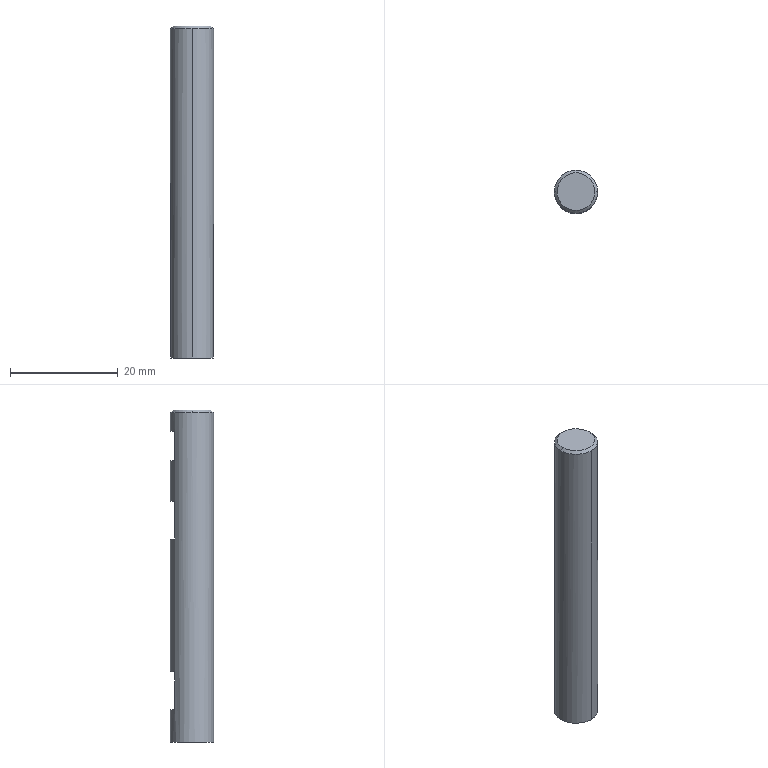Part | NX | 1 solid | 23 faces | box 8 x 8 x 61.5 mm | volume 2929 mm3 | plane 11 | cylinder 6 | cone 6 | commonest cylinder face diameters 3.3 x4 8 x2
STEP:
#1=CARTESIAN_POINT('',(-190.,192.7,-6.3));
#2=VERTEX_POINT('',#1);
#3=CARTESIAN_POINT('',(-194.,196.7,-6.3));
#4=VERTEX_POINT('',#3);
#5=CARTESIAN_POINT('',(-190.,196.7,-6.3));
#6=DIRECTION('',(0.,0.,-1.));
#7=DIRECTION('',(-1.,0.,0.));
#8=AXIS2_PLACEMENT_3D('',#5,#6,#7);
#9=CIRCLE('',#8,4.);
#10=EDGE_CURVE('',#2,#4,#9,.T.);
#11=ORIENTED_EDGE('',*,*,#10,.T.);
#12=CARTESIAN_POINT('',(-190.,200.7,-6.3));
#13=VERTEX_POINT('',#12);
#14=CARTESIAN_POINT('',(-190.,196.7,-6.3));
#15=DIRECTION('',(0.,0.,-1.));
#16=DIRECTION('',(-1.,0.,0.));
#17=AXIS2_PLACEMENT_3D('',#14,#15,#16);
#18=CIRCLE('',#17,4.);
#19=EDGE_CURVE('',#4,#13,#18,.T.);
#20=ORIENTED_EDGE('',*,*,#19,.T.);
#21=CARTESIAN_POINT('',(-190.,200.7,-9.7));
#22=VERTEX_POINT('',#21);
#23=CARTESIAN_POINT('',(-190.,200.7,-55.8));
#24=DIRECTION('',(0.,0.,1.));
#25=VECTOR('',#24,1000.);
#26=LINE('',#23,#25);
#27=EDGE_CURVE('',#13,#22,#26,.F.);
#28=ORIENTED_EDGE('',*,*,#27,.T.);
#29=CARTESIAN_POINT('',(-192.4,199.9,-9.7));
#30=VERTEX_POINT('',#29);
#31=CARTESIAN_POINT('',(-190.,196.7,-9.7));
#32=DIRECTION('',(0.,0.,1.));
#33=DIRECTION('',(0.,-1.,0.));
#34=AXIS2_PLACEMENT_3D('',#31,#32,#33);
#35=CIRCLE('',#34,4.);
#36=EDGE_CURVE('',#22,#30,#35,.T.);
#37=ORIENTED_EDGE('',*,*,#36,.T.);
#38=CARTESIAN_POINT('',(-192.4,199.9,-15.2));
#39=VERTEX_POINT('',#38);
#40=CARTESIAN_POINT('',(-192.4,199.9,-55.8));
#41=DIRECTION('',(0.,0.,1.));
#42=VECTOR('',#41,1000.);
#43=LINE('',#40,#42);
#44=EDGE_CURVE('',#39,#30,#43,.T.);
#45=ORIENTED_EDGE('',*,*,#44,.F.);
#46=CARTESIAN_POINT('',(-190.,200.7,-15.2));
#47=VERTEX_POINT('',#46);
#48=CARTESIAN_POINT('',(-190.,196.7,-15.2));
#49=DIRECTION('',(0.,0.,1.));
#50=DIRECTION('',(0.,-1.,0.));
#51=AXIS2_PLACEMENT_3D('',#48,#49,#50);
#52=CIRCLE('',#51,4.);
#53=EDGE_CURVE('',#47,#39,#52,.T.);
#54=ORIENTED_EDGE('',*,*,#53,.F.);
#55=CARTESIAN_POINT('',(-190.,200.7,-22.7));
#56=VERTEX_POINT('',#55);
#57=CARTESIAN_POINT('',(-190.,200.7,-55.8));
#58=DIRECTION('',(0.,0.,1.));
#59=VECTOR('',#58,1000.);
#60=LINE('',#57,#59);
#61=EDGE_CURVE('',#56,#47,#60,.T.);
#62=ORIENTED_EDGE('',*,*,#61,.F.);
#63=CARTESIAN_POINT('',(-192.4,199.9,-22.7));
#64=VERTEX_POINT('',#63);
#65=CARTESIAN_POINT('',(-190.,196.7,-22.7));
#66=DIRECTION('',(0.,0.,1.));
#67=DIRECTION('',(0.,-1.,0.));
#68=AXIS2_PLACEMENT_3D('',#65,#66,#67);
#69=CIRCLE('',#68,4.);
#70=EDGE_CURVE('',#56,#64,#69,.T.);
#71=ORIENTED_EDGE('',*,*,#70,.T.);
#72=CARTESIAN_POINT('',(-192.4,199.9,-29.7));
#73=VERTEX_POINT('',#72);
#74=CARTESIAN_POINT('',(-192.4,199.9,-55.8));
#75=DIRECTION('',(0.,0.,1.));
#76=VECTOR('',#75,1000.);
#77=LINE('',#74,#76);
#78=EDGE_CURVE('',#73,#64,#77,.T.);
#79=ORIENTED_EDGE('',*,*,#78,.F.);
#80=CARTESIAN_POINT('',(-190.,200.7,-29.7));
#81=VERTEX_POINT('',#80);
#82=CARTESIAN_POINT('',(-190.,196.7,-29.7));
#83=DIRECTION('',(0.,0.,1.));
#84=DIRECTION('',(0.,-1.,0.));
#85=AXIS2_PLACEMENT_3D('',#82,#83,#84);
#86=CIRCLE('',#85,4.);
#87=EDGE_CURVE('',#81,#73,#86,.T.);
#88=ORIENTED_EDGE('',*,*,#87,.F.);
#89=CARTESIAN_POINT('',(-190.,200.7,-54.3));
#90=VERTEX_POINT('',#89);
#91=CARTESIAN_POINT('',(-190.,200.7,-55.8));
#92=DIRECTION('',(0.,0.,1.));
#93=VECTOR('',#92,1000.);
#94=LINE('',#91,#93);
#95=EDGE_CURVE('',#90,#81,#94,.T.);
#96=ORIENTED_EDGE('',*,*,#95,.F.);
#97=CARTESIAN_POINT('',(-192.4,199.9,-54.3));
#98=VERTEX_POINT('',#97);
#99=CARTESIAN_POINT('',(-190.,196.7,-54.3));
#100=DIRECTION('',(0.,0.,1.));
#101=DIRECTION('',(0.,-1.,0.));
#102=AXIS2_PLACEMENT_3D('',#99,#100,#101);
#103=CIRCLE('',#102,4.);
#104=EDGE_CURVE('',#90,#98,#103,.T.);
#105=ORIENTED_EDGE('',*,*,#104,.T.);
#106=CARTESIAN_POINT('',(-192.4,199.9,-61.3));
#107=VERTEX_POINT('',#106);
#108=CARTESIAN_POINT('',(-192.4,199.9,-55.8));
#109=DIRECTION('',(0.,0.,1.));
#110=VECTOR('',#109,1000.);
#111=LINE('',#108,#110);
#112=EDGE_CURVE('',#107,#98,#111,.T.);
#113=ORIENTED_EDGE('',*,*,#112,.F.);
#114=CARTESIAN_POINT('',(-190.,200.7,-61.3));
#115=VERTEX_POINT('',#114);
#116=CARTESIAN_POINT('',(-190.,196.7,-61.3));
#117=DIRECTION('',(0.,0.,1.));
#118=DIRECTION('',(0.,-1.,0.));
#119=AXIS2_PLACEMENT_3D('',#116,#117,#118);
#120=CIRCLE('',#119,4.);
#121=EDGE_CURVE('',#115,#107,#120,.T.);
#122=ORIENTED_EDGE('',*,*,#121,.F.);
#123=CARTESIAN_POINT('',(-190.,200.7,-67.3));
#124=VERTEX_POINT('',#123);
#125=CARTESIAN_POINT('',(-190.,200.7,-55.8));
#126=DIRECTION('',(0.,0.,1.));
#127=VECTOR('',#126,1000.);
#128=LINE('',#125,#127);
#129=EDGE_CURVE('',#124,#115,#128,.T.);
#130=ORIENTED_EDGE('',*,*,#129,.F.);
#131=CARTESIAN_POINT('',(-190.,192.7,-67.3));
#132=VERTEX_POINT('',#131);
#133=CARTESIAN_POINT('',(-190.,196.7,-67.3));
#134=DIRECTION('',(0.,0.,1.));
#135=DIRECTION('',(0.,-1.,0.));
#136=AXIS2_PLACEMENT_3D('',#133,#134,#135);
#137=CIRCLE('',#136,4.);
#138=EDGE_CURVE('',#124,#132,#137,.T.);
#139=ORIENTED_EDGE('',*,*,#138,.T.);
#140=CARTESIAN_POINT('',(-190.,192.7,-55.8));
#141=DIRECTION('',(0.,0.,1.));
#142=VECTOR('',#141,1000.);
#143=LINE('',#140,#142);
#144=EDGE_CURVE('',#2,#132,#143,.F.);
#145=ORIENTED_EDGE('',*,*,#144,.F.);
#146=EDGE_LOOP('',(#11,#20,#28,#37,#45,#54,#62,#71,#79,#88,#96,#105,#113,#122,#130,#139,#145));
#147=FACE_BOUND('',#146,.T.);
#148=CARTESIAN_POINT('',(-190.,196.7,-55.8));
#149=DIRECTION('',(0.,0.,1.));
#150=DIRECTION('',(0.,-1.,0.));
#151=AXIS2_PLACEMENT_3D('',#148,#149,#150);
#152=CYLINDRICAL_SURFACE('',#151,4.);
#153=ADVANCED_FACE('',(#147),#152,.T.);
#154=CARTESIAN_POINT('',(-193.5,196.7,-5.8));
#155=VERTEX_POINT('',#154);
#156=CARTESIAN_POINT('',(-186.5,196.7,-5.8));
#157=VERTEX_POINT('',#156);
#158=CARTESIAN_POINT('',(-190.,196.7,-5.8));
#159=DIRECTION('',(0.,0.,1.));
#160=DIRECTION('',(1.,0.,0.));
#161=AXIS2_PLACEMENT_3D('',#158,#159,#160);
#162=CIRCLE('',#161,3.5);
#163=EDGE_CURVE('',#155,#157,#162,.T.);
#164=ORIENTED_EDGE('',*,*,#163,.F.);
#165=CARTESIAN_POINT('',(-193.5,196.7,-5.8));
#166=DIRECTION('',(-0.7071,0.,-0.7071));
#167=VECTOR('',#166,1000.);
#168=LINE('',#165,#167);
#169=EDGE_CURVE('',#4,#155,#168,.F.);
#170=ORIENTED_EDGE('',*,*,#169,.F.);
#171=ORIENTED_EDGE('',*,*,#10,.F.);
#172=CARTESIAN_POINT('',(-186.,196.7,-6.3));
#173=VERTEX_POINT('',#172);
#174=CARTESIAN_POINT('',(-190.,196.7,-6.3));
#175=DIRECTION('',(0.,0.,-1.));
#176=DIRECTION('',(-1.,0.,0.));
#177=AXIS2_PLACEMENT_3D('',#174,#175,#176);
#178=CIRCLE('',#177,4.);
#179=EDGE_CURVE('',#173,#2,#178,.T.);
#180=ORIENTED_EDGE('',*,*,#179,.F.);
#181=CARTESIAN_POINT('',(-186.5,196.7,-5.8));
#182=DIRECTION('',(0.7071,0.,-0.7071));
#183=VECTOR('',#182,1000.);
#184=LINE('',#181,#183);
#185=EDGE_CURVE('',#173,#157,#184,.F.);
#186=ORIENTED_EDGE('',*,*,#185,.T.);
#187=EDGE_LOOP('',(#164,#170,#171,#180,#186));
#188=FACE_BOUND('',#187,.T.);
#189=CARTESIAN_POINT('',(-190.,196.7,-5.8));
#190=DIRECTION('',(0.,0.,-1.));
#191=DIRECTION('',(-1.,0.,0.));
#192=AXIS2_PLACEMENT_3D('',#189,#190,#191);
#193=CONICAL_SURFACE('',#192,3.5,0.7854);
#194=ADVANCED_FACE('',(#188),#193,.T.);
#195=ORIENTED_EDGE('',*,*,#163,.T.);
#196=CARTESIAN_POINT('',(-190.,196.7,-5.8));
#197=DIRECTION('',(0.,0.,1.));
#198=DIRECTION('',(1.,0.,0.));
#199=AXIS2_PLACEMENT_3D('',#196,#197,#198);
#200=CIRCLE('',#199,3.5);
#201=EDGE_CURVE('',#157,#155,#200,.T.);
#202=ORIENTED_EDGE('',*,*,#201,.T.);
#203=EDGE_LOOP('',(#195,#202));
#204=FACE_BOUND('',#203,.T.);
#205=CARTESIAN_POINT('',(-181.498,197.784,-5.8));
#206=DIRECTION('',(0.,0.,-1.));
#207=DIRECTION('',(-1.,0.,0.));
#208=AXIS2_PLACEMENT_3D('',#205,#206,#207);
#209=PLANE('',#208);
#210=ADVANCED_FACE('',(#204),#209,.F.);
#211=ORIENTED_EDGE('',*,*,#70,.F.);
#212=CARTESIAN_POINT('',(-187.6,199.9,-22.7));
#213=VERTEX_POINT('',#212);
#214=CARTESIAN_POINT('',(-190.,196.7,-22.7));
#215=DIRECTION('',(0.,0.,1.));
#216=DIRECTION('',(0.,-1.,0.));
#217=AXIS2_PLACEMENT_3D('',#214,#215,#216);
#218=CIRCLE('',#217,4.);
#219=EDGE_CURVE('',#213,#56,#218,.T.);
#220=ORIENTED_EDGE('',*,*,#219,.F.);
#221=CARTESIAN_POINT('',(0.,199.9,-22.7));
#222=DIRECTION('',(-1.,0.,0.));
#223=VECTOR('',#222,1000.);
#224=LINE('',#221,#223);
#225=EDGE_CURVE('',#213,#64,#224,.T.);
#226=ORIENTED_EDGE('',*,*,#225,.T.);
#227=EDGE_LOOP('',(#211,#220,#226));
#228=FACE_BOUND('',#227,.T.);
#229=CARTESIAN_POINT('',(-190.,208.7,-22.7));
#230=DIRECTION('',(0.,0.,1.));
#231=DIRECTION('',(1.,0.,0.));
#232=AXIS2_PLACEMENT_3D('',#229,#230,#231);
#233=PLANE('',#232);
#234=ADVANCED_FACE('',(#228),#233,.F.);
#235=ORIENTED_EDGE('',*,*,#138,.F.);
#236=CARTESIAN_POINT('',(-190.,196.7,-67.3));
#237=DIRECTION('',(0.,0.,1.));
#238=DIRECTION('',(0.,-1.,0.));
#239=AXIS2_PLACEMENT_3D('',#236,#237,#238);
#240=CIRCLE('',#239,4.);
#241=EDGE_CURVE('',#132,#124,#240,.T.);
#242=ORIENTED_EDGE('',*,*,#241,.F.);
#243=EDGE_LOOP('',(#235,#242));
#244=FACE_BOUND('',#243,.T.);
#245=CARTESIAN_POINT('',(-187.685,196.7,-67.3));
#246=VERTEX_POINT('',#245);
#247=CARTESIAN_POINT('',(-192.315,196.7,-67.3));
#248=VERTEX_POINT('',#247);
#249=CARTESIAN_POINT('',(-190.,196.7,-67.3));
#250=DIRECTION('',(0.,0.,-1.));
#251=DIRECTION('',(-1.,0.,0.));
#252=AXIS2_PLACEMENT_3D('',#249,#250,#251);
#253=CIRCLE('',#252,2.315);
#254=EDGE_CURVE('',#246,#248,#253,.T.);
#255=ORIENTED_EDGE('',*,*,#254,.F.);
#256=CARTESIAN_POINT('',(-190.,196.7,-67.3));
#257=DIRECTION('',(0.,0.,-1.));
#258=DIRECTION('',(-1.,0.,0.));
#259=AXIS2_PLACEMENT_3D('',#256,#257,#258);
#260=CIRCLE('',#259,2.315);
#261=EDGE_CURVE('',#248,#246,#260,.T.);
#262=ORIENTED_EDGE('',*,*,#261,.F.);
#263=EDGE_LOOP('',(#255,#262));
#264=FACE_BOUND('',#263,.T.);
#265=CARTESIAN_POINT('',(-181.498,197.784,-67.3));
#266=DIRECTION('',(0.,0.,-1.));
#267=DIRECTION('',(-1.,0.,0.));
#268=AXIS2_PLACEMENT_3D('',#265,#266,#267);
#269=PLANE('',#268);
#270=ADVANCED_FACE('',(#244,#264),#269,.T.);
#271=ORIENTED_EDGE('',*,*,#121,.T.);
#272=CARTESIAN_POINT('',(-187.6,199.9,-61.3));
#273=VERTEX_POINT('',#272);
#274=CARTESIAN_POINT('',(0.,199.9,-61.3));
#275=DIRECTION('',(-1.,0.,0.));
#276=VECTOR('',#275,1000.);
#277=LINE('',#274,#276);
#278=EDGE_CURVE('',#273,#107,#277,.T.);
#279=ORIENTED_EDGE('',*,*,#278,.F.);
#280=CARTESIAN_POINT('',(-190.,196.7,-61.3));
#281=DIRECTION('',(0.,0.,1.));
#282=DIRECTION('',(0.,-1.,0.));
#283=AXIS2_PLACEMENT_3D('',#280,#281,#282);
#284=CIRCLE('',#283,4.);
#285=EDGE_CURVE('',#273,#115,#284,.T.);
#286=ORIENTED_EDGE('',*,*,#285,.T.);
#287=EDGE_LOOP('',(#271,#279,#286));
#288=FACE_BOUND('',#287,.T.);
#289=CARTESIAN_POINT('',(-190.,208.7,-61.3));
#290=DIRECTION('',(0.,0.,-1.));
#291=DIRECTION('',(0.,-1.,0.));
#292=AXIS2_PLACEMENT_3D('',#289,#290,#291);
#293=PLANE('',#292);
#294=ADVANCED_FACE('',(#288),#293,.F.);
#295=ORIENTED_EDGE('',*,*,#36,.F.);
#296=CARTESIAN_POINT('',(-187.6,199.9,-9.7));
#297=VERTEX_POINT('',#296);
#298=CARTESIAN_POINT('',(-190.,196.7,-9.7));
#299=DIRECTION('',(0.,0.,1.));
#300=DIRECTION('',(0.,-1.,0.));
#301=AXIS2_PLACEMENT_3D('',#298,#299,#300);
#302=CIRCLE('',#301,4.);
#303=EDGE_CURVE('',#297,#22,#302,.T.);
#304=ORIENTED_EDGE('',*,*,#303,.F.);
#305=CARTESIAN_POINT('',(-181.498,199.9,-9.7));
#306=DIRECTION('',(1.,0.,0.));
#307=VECTOR('',#306,1000.);
#308=LINE('',#305,#307);
#309=EDGE_CURVE('',#30,#297,#308,.T.);
#310=ORIENTED_EDGE('',*,*,#309,.F.);
#311=EDGE_LOOP('',(#295,#304,#310));
#312=FACE_BOUND('',#311,.T.);
#313=CARTESIAN_POINT('',(-185.645,200.992,-9.7));
#314=DIRECTION('',(0.,0.,1.));
#315=DIRECTION('',(1.,0.,0.));
#316=AXIS2_PLACEMENT_3D('',#313,#314,#315);
#317=PLANE('',#316);
#318=ADVANCED_FACE('',(#312),#317,.F.);
#319=CARTESIAN_POINT('',(-187.6,199.9,-15.2));
#320=VERTEX_POINT('',#319);
#321=CARTESIAN_POINT('',(-181.498,199.9,-15.2));
#322=DIRECTION('',(1.,0.,0.));
#323=VECTOR('',#322,1000.);
#324=LINE('',#321,#323);
#325=EDGE_CURVE('',#39,#320,#324,.T.);
#326=ORIENTED_EDGE('',*,*,#325,.T.);
#327=CARTESIAN_POINT('',(-190.,196.7,-15.2));
#328=DIRECTION('',(0.,0.,1.));
#329=DIRECTION('',(0.,-1.,0.));
#330=AXIS2_PLACEMENT_3D('',#327,#328,#329);
#331=CIRCLE('',#330,4.);
#332=EDGE_CURVE('',#320,#47,#331,.T.);
#333=ORIENTED_EDGE('',*,*,#332,.T.);
#334=ORIENTED_EDGE('',*,*,#53,.T.);
#335=EDGE_LOOP('',(#326,#333,#334));
#336=FACE_BOUND('',#335,.T.);
#337=CARTESIAN_POINT('',(-185.645,200.992,-15.2));
#338=DIRECTION('',(0.,0.,1.));
#339=DIRECTION('',(1.,0.,0.));
#340=AXIS2_PLACEMENT_3D('',#337,#338,#339);
#341=PLANE('',#340);
#342=ADVANCED_FACE('',(#336),#341,.T.);
#343=CARTESIAN_POINT('',(-187.6,199.9,-55.8));
#344=DIRECTION('',(0.,0.,1.));
#345=VECTOR('',#344,1000.);
#346=LINE('',#343,#345);
#347=EDGE_CURVE('',#320,#297,#346,.T.);
#348=ORIENTED_EDGE('',*,*,#347,.F.);
#349=ORIENTED_EDGE('',*,*,#325,.F.);
#350=ORIENTED_EDGE('',*,*,#44,.T.);
#351=ORIENTED_EDGE('',*,*,#309,.T.);
#352=EDGE_LOOP('',(#348,#349,#350,#351));
#353=FACE_BOUND('',#352,.T.);
#354=CARTESIAN_POINT('',(-192.646,199.9,-13.2));
#355=DIRECTION('',(0.,-1.,0.));
#356=DIRECTION('',(-1.,0.,0.));
#357=AXIS2_PLACEMENT_3D('',#354,#355,#356);
#358=PLANE('',#357);
#359=ADVANCED_FACE('',(#353),#358,.F.);
#360=ORIENTED_EDGE('',*,*,#104,.F.);
#361=CARTESIAN_POINT('',(-187.6,199.9,-54.3));
#362=VERTEX_POINT('',#361);
#363=CARTESIAN_POINT('',(-190.,196.7,-54.3));
#364=DIRECTION('',(0.,0.,1.));
#365=DIRECTION('',(0.,-1.,0.));
#366=AXIS2_PLACEMENT_3D('',#363,#364,#365);
#367=CIRCLE('',#366,4.);
#368=EDGE_CURVE('',#362,#90,#367,.T.);
#369=ORIENTED_EDGE('',*,*,#368,.F.);
#370=CARTESIAN_POINT('',(0.,199.9,-54.3));
#371=DIRECTION('',(-1.,0.,0.));
#372=VECTOR('',#371,1000.);
#373=LINE('',#370,#372);
#374=EDGE_CURVE('',#362,#98,#373,.T.);
#375=ORIENTED_EDGE('',*,*,#374,.T.);
#376=EDGE_LOOP('',(#360,#369,#375));
#377=FACE_BOUND('',#376,.T.);
#378=CARTESIAN_POINT('',(-190.,208.7,-54.3));
#379=DIRECTION('',(0.,0.,1.));
#380=DIRECTION('',(1.,0.,0.));
#381=AXIS2_PLACEMENT_3D('',#378,#379,#380);
#382=PLANE('',#381);
#383=ADVANCED_FACE('',(#377),#382,.F.);
#384=ORIENTED_EDGE('',*,*,#87,.T.);
#385=CARTESIAN_POINT('',(-187.6,199.9,-29.7));
#386=VERTEX_POINT('',#385);
#387=CARTESIAN_POINT('',(0.,199.9,-29.7));
#388=DIRECTION('',(1.,0.,0.));
#389=VECTOR('',#388,1000.);
#390=LINE('',#387,#389);
#391=EDGE_CURVE('',#73,#386,#390,.T.);
#392=ORIENTED_EDGE('',*,*,#391,.T.);
#393=CARTESIAN_POINT('',(-190.,196.7,-29.7));
#394=DIRECTION('',(0.,0.,1.));
#395=DIRECTION('',(0.,-1.,0.));
#396=AXIS2_PLACEMENT_3D('',#393,#394,#395);
#397=CIRCLE('',#396,4.);
#398=EDGE_CURVE('',#386,#81,#397,.T.);
#399=ORIENTED_EDGE('',*,*,#398,.T.);
#400=EDGE_LOOP('',(#384,#392,#399));
#401=FACE_BOUND('',#400,.T.);
#402=CARTESIAN_POINT('',(-190.,208.7,-29.7));
#403=DIRECTION('',(0.,0.,-1.));
#404=DIRECTION('',(0.,-1.,0.));
#405=AXIS2_PLACEMENT_3D('',#402,#403,#404);
#406=PLANE('',#405);
#407=ADVANCED_FACE('',(#401),#406,.F.);
#408=ORIENTED_EDGE('',*,*,#374,.F.);
#409=CARTESIAN_POINT('',(-187.6,199.9,-55.8));
#410=DIRECTION('',(0.,0.,1.));
#411=VECTOR('',#410,1000.);
#412=LINE('',#409,#411);
#413=EDGE_CURVE('',#273,#362,#412,.T.);
#414=ORIENTED_EDGE('',*,*,#413,.F.);
#415=ORIENTED_EDGE('',*,*,#278,.T.);
#416=ORIENTED_EDGE('',*,*,#112,.T.);
#417=EDGE_LOOP('',(#408,#414,#415,#416));
#418=FACE_BOUND('',#417,.T.);
#419=CARTESIAN_POINT('',(-179.801,199.9,-22.368));
#420=DIRECTION('',(0.,1.,0.));
#421=DIRECTION('',(1.,0.,0.));
#422=AXIS2_PLACEMENT_3D('',#419,#420,#421);
#423=PLANE('',#422);
#424=ADVANCED_FACE('',(#418),#423,.T.);
#425=ORIENTED_EDGE('',*,*,#78,.T.);
#426=ORIENTED_EDGE('',*,*,#225,.F.);
#427=CARTESIAN_POINT('',(-187.6,199.9,-55.8));
#428=DIRECTION('',(0.,0.,1.));
#429=VECTOR('',#428,1000.);
#430=LINE('',#427,#429);
#431=EDGE_CURVE('',#386,#213,#430,.T.);
#432=ORIENTED_EDGE('',*,*,#431,.F.);
#433=ORIENTED_EDGE('',*,*,#391,.F.);
#434=EDGE_LOOP('',(#425,#426,#432,#433));
#435=FACE_BOUND('',#434,.T.);
#436=CARTESIAN_POINT('',(-179.801,199.9,-22.368));
#437=DIRECTION('',(0.,1.,0.));
#438=DIRECTION('',(1.,0.,0.));
#439=AXIS2_PLACEMENT_3D('',#436,#437,#438);
#440=PLANE('',#439);
#441=ADVANCED_FACE('',(#435),#440,.T.);
#442=CARTESIAN_POINT('',(-188.35,196.7,-66.916));
#443=VERTEX_POINT('',#442);
#444=CARTESIAN_POINT('',(-191.65,196.7,-66.916));
#445=VERTEX_POINT('',#444);
#446=CARTESIAN_POINT('',(-190.,196.7,-66.916));
#447=DIRECTION('',(0.,0.,-1.));
#448=DIRECTION('',(-1.,0.,0.));
#449=AXIS2_PLACEMENT_3D('',#446,#447,#448);
#450=CIRCLE('',#449,1.65);
#451=EDGE_CURVE('',#443,#445,#450,.T.);
#452=ORIENTED_EDGE('',*,*,#451,.T.);
#453=CARTESIAN_POINT('',(-191.65,196.7,-59.3));
#454=VERTEX_POINT('',#453);
#455=CARTESIAN_POINT('',(-191.65,196.7,-67.3));
#456=DIRECTION('',(0.,0.,-1.));
#457=VECTOR('',#456,1000.);
#458=LINE('',#455,#457);
#459=EDGE_CURVE('',#445,#454,#458,.F.);
#460=ORIENTED_EDGE('',*,*,#459,.T.);
#461=CARTESIAN_POINT('',(-188.35,196.7,-59.3));
#462=VERTEX_POINT('',#461);
#463=CARTESIAN_POINT('',(-190.,196.7,-59.3));
#464=DIRECTION('',(0.,0.,-1.));
#465=DIRECTION('',(-1.,0.,0.));
#466=AXIS2_PLACEMENT_3D('',#463,#464,#465);
#467=CIRCLE('',#466,1.65);
#468=EDGE_CURVE('',#462,#454,#467,.T.);
#469=ORIENTED_EDGE('',*,*,#468,.F.);
#470=CARTESIAN_POINT('',(-188.35,196.7,-67.3));
#471=DIRECTION('',(0.,0.,-1.));
#472=VECTOR('',#471,1000.);
#473=LINE('',#470,#472);
#474=EDGE_CURVE('',#443,#462,#473,.F.);
#475=ORIENTED_EDGE('',*,*,#474,.F.);
#476=EDGE_LOOP('',(#452,#460,#469,#475));
#477=FACE_BOUND('',#476,.T.);
#478=CARTESIAN_POINT('',(-190.,196.7,-67.3));
#479=DIRECTION('',(0.,0.,-1.));
#480=DIRECTION('',(-1.,0.,0.));
#481=AXIS2_PLACEMENT_3D('',#478,#479,#480);
#482=CYLINDRICAL_SURFACE('',#481,1.65);
#483=ADVANCED_FACE('',(#477),#482,.F.);
#484=ORIENTED_EDGE('',*,*,#468,.T.);
#485=CARTESIAN_POINT('',(-191.65,196.7,-55.1));
#486=VERTEX_POINT('',#485);
#487=CARTESIAN_POINT('',(-191.65,196.7,-67.3));
#488=DIRECTION('',(0.,0.,-1.));
#489=VECTOR('',#488,1000.);
#490=LINE('',#487,#489);
#491=EDGE_CURVE('',#454,#486,#490,.F.);
#492=ORIENTED_EDGE('',*,*,#491,.T.);
#493=CARTESIAN_POINT('',(-188.35,196.7,-55.1));
#494=VERTEX_POINT('',#493);
#495=CARTESIAN_POINT('',(-190.,196.7,-55.1));
#496=DIRECTION('',(0.,0.,-1.));
#497=DIRECTION('',(-1.,0.,0.));
#498=AXIS2_PLACEMENT_3D('',#495,#496,#497);
#499=CIRCLE('',#498,1.65);
#500=EDGE_CURVE('',#494,#486,#499,.T.);
#501=ORIENTED_EDGE('',*,*,#500,.F.);
#502=CARTESIAN_POINT('',(-188.35,196.7,-67.3));
#503=DIRECTION('',(0.,0.,-1.));
#504=VECTOR('',#503,1000.);
#505=LINE('',#502,#504);
#506=EDGE_CURVE('',#462,#494,#505,.F.);
#507=ORIENTED_EDGE('',*,*,#506,.F.);
#508=EDGE_LOOP('',(#484,#492,#501,#507));
#509=FACE_BOUND('',#508,.T.);
#510=CARTESIAN_POINT('',(-190.,196.7,-67.3));
#511=DIRECTION('',(0.,0.,-1.));
#512=DIRECTION('',(-1.,0.,0.));
#513=AXIS2_PLACEMENT_3D('',#510,#511,#512);
#514=CYLINDRICAL_SURFACE('',#513,1.65);
#515=ADVANCED_FACE('',(#509),#514,.F.);
#516=ORIENTED_EDGE('',*,*,#500,.T.);
#517=CARTESIAN_POINT('',(-190.,196.7,-54.109));
#518=VERTEX_POINT('',#517);
#519=CARTESIAN_POINT('',(-191.65,196.7,-55.1));
#520=DIRECTION('',(-0.8572,0.,-0.515));
#521=VECTOR('',#520,1000.);
#522=LINE('',#519,#521);
#523=EDGE_CURVE('',#518,#486,#522,.T.);
#524=ORIENTED_EDGE('',*,*,#523,.F.);
#525=CARTESIAN_POINT('',(-188.35,196.7,-55.1));
#526=DIRECTION('',(0.8572,0.,-0.515));
#527=VECTOR('',#526,1000.);
#528=LINE('',#525,#527);
#529=EDGE_CURVE('',#518,#494,#528,.T.);
#530=ORIENTED_EDGE('',*,*,#529,.T.);
#531=EDGE_LOOP('',(#516,#524,#530));
#532=FACE_BOUND('',#531,.T.);
#533=CARTESIAN_POINT('',(-190.,196.7,-55.1));
#534=DIRECTION('',(0.,0.,-1.));
#535=DIRECTION('',(-1.,0.,0.));
#536=AXIS2_PLACEMENT_3D('',#533,#534,#535);
#537=CONICAL_SURFACE('',#536,1.65,1.03);
#538=ADVANCED_FACE('',(#532),#537,.F.);
#539=ORIENTED_EDGE('',*,*,#451,.F.);
#540=CARTESIAN_POINT('',(-188.35,196.7,-66.916));
#541=DIRECTION('',(0.866,0.,-0.5));
#542=VECTOR('',#541,1000.);
#543=LINE('',#540,#542);
#544=EDGE_CURVE('',#246,#443,#543,.F.);
#545=ORIENTED_EDGE('',*,*,#544,.F.);
#546=ORIENTED_EDGE('',*,*,#254,.T.);
#547=CARTESIAN_POINT('',(-191.65,196.7,-66.916));
#548=DIRECTION('',(-0.866,0.,-0.5));
#549=VECTOR('',#548,1000.);
#550=LINE('',#547,#549);
#551=EDGE_CURVE('',#248,#445,#550,.F.);
#552=ORIENTED_EDGE('',*,*,#551,.T.);
#553=EDGE_LOOP('',(#539,#545,#546,#552));
#554=FACE_BOUND('',#553,.T.);
#555=CARTESIAN_POINT('',(-190.,196.7,-66.916));
#556=DIRECTION('',(0.,0.,-1.));
#557=DIRECTION('',(-1.,0.,0.));
#558=AXIS2_PLACEMENT_3D('',#555,#556,#557);
#559=CONICAL_SURFACE('',#558,1.65,1.047);
#560=ADVANCED_FACE('',(#554),#559,.F.);
#561=ORIENTED_EDGE('',*,*,#169,.T.);
#562=ORIENTED_EDGE('',*,*,#201,.F.);
#563=ORIENTED_EDGE('',*,*,#185,.F.);
#564=CARTESIAN_POINT('',(-190.,196.7,-6.3));
#565=DIRECTION('',(0.,0.,-1.));
#566=DIRECTION('',(-1.,0.,0.));
#567=AXIS2_PLACEMENT_3D('',#564,#565,#566);
#568=CIRCLE('',#567,4.);
#569=EDGE_CURVE('',#13,#173,#568,.T.);
#570=ORIENTED_EDGE('',*,*,#569,.F.);
#571=ORIENTED_EDGE('',*,*,#19,.F.);
#572=EDGE_LOOP('',(#561,#562,#563,#570,#571));
#573=FACE_BOUND('',#572,.T.);
#574=CARTESIAN_POINT('',(-190.,196.7,-5.8));
#575=DIRECTION('',(0.,0.,-1.));
#576=DIRECTION('',(-1.,0.,0.));
#577=AXIS2_PLACEMENT_3D('',#574,#575,#576);
#578=CONICAL_SURFACE('',#577,3.5,0.7854);
#579=ADVANCED_FACE('',(#573),#578,.T.);
#580=ORIENTED_EDGE('',*,*,#144,.T.);
#581=ORIENTED_EDGE('',*,*,#241,.T.);
#582=ORIENTED_EDGE('',*,*,#129,.T.);
#583=ORIENTED_EDGE('',*,*,#285,.F.);
#584=ORIENTED_EDGE('',*,*,#413,.T.);
#585=ORIENTED_EDGE('',*,*,#368,.T.);
#586=ORIENTED_EDGE('',*,*,#95,.T.);
#587=ORIENTED_EDGE('',*,*,#398,.F.);
#588=ORIENTED_EDGE('',*,*,#431,.T.);
#589=ORIENTED_EDGE('',*,*,#219,.T.);
#590=ORIENTED_EDGE('',*,*,#61,.T.);
#591=ORIENTED_EDGE('',*,*,#332,.F.);
#592=ORIENTED_EDGE('',*,*,#347,.T.);
#593=ORIENTED_EDGE('',*,*,#303,.T.);
#594=ORIENTED_EDGE('',*,*,#27,.F.);
#595=ORIENTED_EDGE('',*,*,#569,.T.);
#596=ORIENTED_EDGE('',*,*,#179,.T.);
#597=EDGE_LOOP('',(#580,#581,#582,#583,#584,#585,#586,#587,#588,#589,#590,#591,#592,#593,#594,#595,#596));
#598=FACE_BOUND('',#597,.T.);
#599=CARTESIAN_POINT('',(-190.,196.7,-55.8));
#600=DIRECTION('',(0.,0.,1.));
#601=DIRECTION('',(0.,-1.,0.));
#602=AXIS2_PLACEMENT_3D('',#599,#600,#601);
#603=CYLINDRICAL_SURFACE('',#602,4.);
#604=ADVANCED_FACE('',(#598),#603,.T.);
#605=ORIENTED_EDGE('',*,*,#529,.F.);
#606=ORIENTED_EDGE('',*,*,#523,.T.);
#607=CARTESIAN_POINT('',(-190.,196.7,-55.1));
#608=DIRECTION('',(0.,0.,-1.));
#609=DIRECTION('',(-1.,0.,0.));
#610=AXIS2_PLACEMENT_3D('',#607,#608,#609);
#611=CIRCLE('',#610,1.65);
#612=EDGE_CURVE('',#486,#494,#611,.T.);
#613=ORIENTED_EDGE('',*,*,#612,.T.);
#614=EDGE_LOOP('',(#605,#606,#613));
#615=FACE_BOUND('',#614,.T.);
#616=CARTESIAN_POINT('',(-190.,196.7,-55.1));
#617=DIRECTION('',(0.,0.,-1.));
#618=DIRECTION('',(-1.,0.,0.));
#619=AXIS2_PLACEMENT_3D('',#616,#617,#618);
#620=CONICAL_SURFACE('',#619,1.65,1.03);
#621=ADVANCED_FACE('',(#615),#620,.F.);
#622=ORIENTED_EDGE('',*,*,#491,.F.);
#623=CARTESIAN_POINT('',(-190.,196.7,-59.3));
#624=DIRECTION('',(0.,0.,-1.));
#625=DIRECTION('',(-1.,0.,0.));
#626=AXIS2_PLACEMENT_3D('',#623,#624,#625);
#627=CIRCLE('',#626,1.65);
#628=EDGE_CURVE('',#454,#462,#627,.T.);
#629=ORIENTED_EDGE('',*,*,#628,.T.);
#630=ORIENTED_EDGE('',*,*,#506,.T.);
#631=ORIENTED_EDGE('',*,*,#612,.F.);
#632=EDGE_LOOP('',(#622,#629,#630,#631));
#633=FACE_BOUND('',#632,.T.);
#634=CARTESIAN_POINT('',(-190.,196.7,-67.3));
#635=DIRECTION('',(0.,0.,-1.));
#636=DIRECTION('',(-1.,0.,0.));
#637=AXIS2_PLACEMENT_3D('',#634,#635,#636);
#638=CYLINDRICAL_SURFACE('',#637,1.65);
#639=ADVANCED_FACE('',(#633),#638,.F.);
#640=ORIENTED_EDGE('',*,*,#459,.F.);
#641=CARTESIAN_POINT('',(-190.,196.7,-66.916));
#642=DIRECTION('',(0.,0.,-1.));
#643=DIRECTION('',(-1.,0.,0.));
#644=AXIS2_PLACEMENT_3D('',#641,#642,#643);
#645=CIRCLE('',#644,1.65);
#646=EDGE_CURVE('',#445,#443,#645,.T.);
#647=ORIENTED_EDGE('',*,*,#646,.T.);
#648=ORIENTED_EDGE('',*,*,#474,.T.);
#649=ORIENTED_EDGE('',*,*,#628,.F.);
#650=EDGE_LOOP('',(#640,#647,#648,#649));
#651=FACE_BOUND('',#650,.T.);
#652=CARTESIAN_POINT('',(-190.,196.7,-67.3));
#653=DIRECTION('',(0.,0.,-1.));
#654=DIRECTION('',(-1.,0.,0.));
#655=AXIS2_PLACEMENT_3D('',#652,#653,#654);
#656=CYLINDRICAL_SURFACE('',#655,1.65);
#657=ADVANCED_FACE('',(#651),#656,.F.);
#658=ORIENTED_EDGE('',*,*,#551,.F.);
#659=ORIENTED_EDGE('',*,*,#261,.T.);
#660=ORIENTED_EDGE('',*,*,#544,.T.);
#661=ORIENTED_EDGE('',*,*,#646,.F.);
#662=EDGE_LOOP('',(#658,#659,#660,#661));
#663=FACE_BOUND('',#662,.T.);
#664=CARTESIAN_POINT('',(-190.,196.7,-66.916));
#665=DIRECTION('',(0.,0.,-1.));
#666=DIRECTION('',(-1.,0.,0.));
#667=AXIS2_PLACEMENT_3D('',#664,#665,#666);
#668=CONICAL_SURFACE('',#667,1.65,1.047);
#669=ADVANCED_FACE('',(#663),#668,.F.);
#670=CLOSED_SHELL('',(#153,#194,#210,#234,#270,#294,#318,#342,#359,#383,#407,#424,#441,#483,#515,#538,#560,#579,#604,#621,#639,#657,#669));
#671=MANIFOLD_SOLID_BREP('',#670);
#672=(LENGTH_UNIT()NAMED_UNIT(*)SI_UNIT(.MILLI.,.METRE.));
#673=UNCERTAINTY_MEASURE_WITH_UNIT(LENGTH_MEASURE(0.00001),#672,'','');
#674=(NAMED_UNIT(*)PLANE_ANGLE_UNIT()SI_UNIT($,.RADIAN.));
#675=(NAMED_UNIT(*)SI_UNIT($,.STERADIAN.)SOLID_ANGLE_UNIT());
#676=(GEOMETRIC_REPRESENTATION_CONTEXT(3)GLOBAL_UNCERTAINTY_ASSIGNED_CONTEXT((#673))GLOBAL_UNIT_ASSIGNED_CONTEXT((#672,#674,#675))REPRESENTATION_CONTEXT('',''));
#677=ADVANCED_BREP_SHAPE_REPRESENTATION('',(#671),#676);